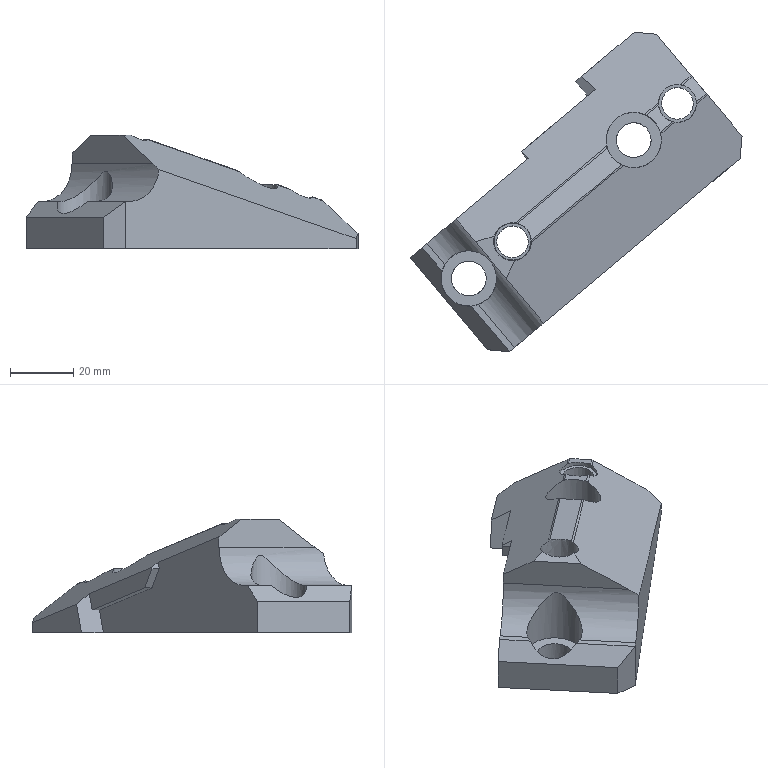Part | NX | features solid 2 | 1 solid | 43 faces | box 104.861 x 100.899 x 36 mm | volume 85049 mm3 | plane 34 | cylinder 7 | spline 2 | commonest cylinder face diameters 10 x2 11 x2 17.5 x2 24 x1